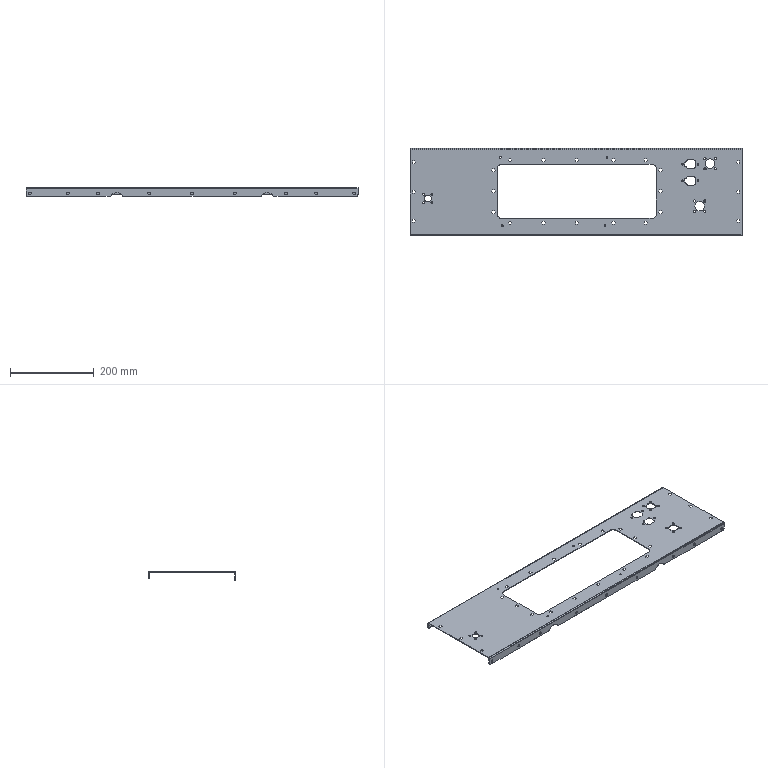Part | NX | features BREP 1 | 1 solid | 312 faces | box 795 x 208.3 x 21.5 mm | volume 208004 mm3 | plane 208 | cylinder 104 | commonest cylinder face diameters 6.5 x18 4.5 x16 5.4 x16 4 x12 12 x8 12.2 x8